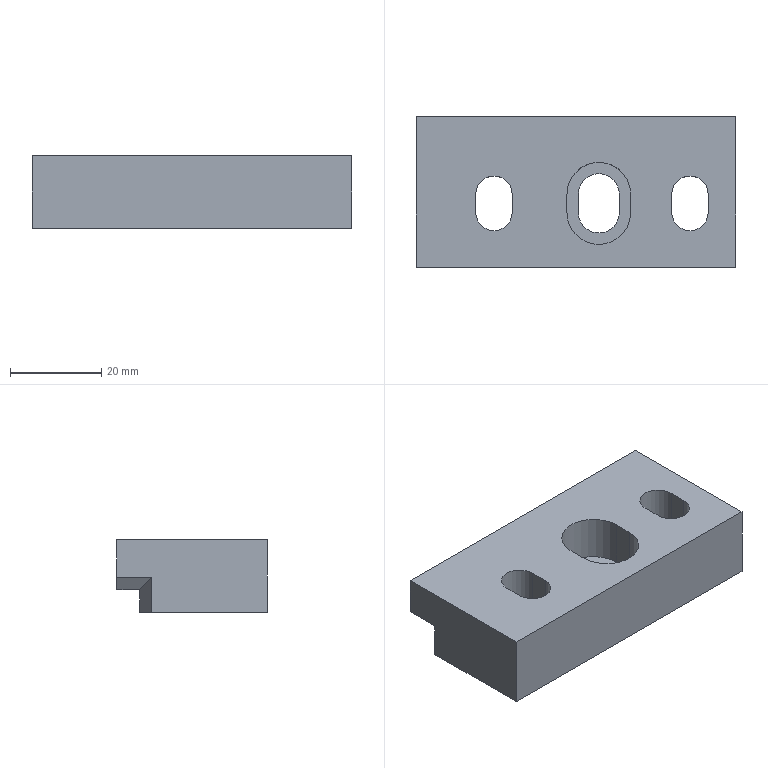Part | STEP file | 1 solid | 29 faces | box 70 x 33 x 16 mm | volume 29565 mm3 | plane 21 | cylinder 8 | commonest cylinder face diameters 8 x4 9 x2 14 x2
STEP:
#1=CARTESIAN_POINT('',(-300.,-103.979,-2.));
#2=VERTEX_POINT('',#1);
#3=CARTESIAN_POINT('',(-300.,-103.979,5.679));
#4=VERTEX_POINT('',#3);
#5=CARTESIAN_POINT('',(-300.,-103.979,-18.));
#6=DIRECTION('',(0.,0.,1.));
#7=VECTOR('',#6,1.);
#8=LINE('',#5,#7);
#9=EDGE_CURVE('',#2,#4,#8,.T.);
#10=ORIENTED_EDGE('',*,*,#9,.T.);
#11=CARTESIAN_POINT('',(-300.,-96.3,5.679));
#12=VERTEX_POINT('',#11);
#13=CARTESIAN_POINT('',(-300.,-129.3,5.679));
#14=DIRECTION('',(0.,1.,0.));
#15=VECTOR('',#14,1.);
#16=LINE('',#13,#15);
#17=EDGE_CURVE('',#4,#12,#16,.T.);
#18=ORIENTED_EDGE('',*,*,#17,.T.);
#19=CARTESIAN_POINT('',(-300.,-96.3,14.));
#20=VERTEX_POINT('',#19);
#21=CARTESIAN_POINT('',(-300.,-96.3,-2.));
#22=DIRECTION('',(0.,0.,1.));
#23=VECTOR('',#22,1.);
#24=LINE('',#21,#23);
#25=EDGE_CURVE('',#12,#20,#24,.T.);
#26=ORIENTED_EDGE('',*,*,#25,.T.);
#27=CARTESIAN_POINT('',(-300.,-129.3,14.));
#28=VERTEX_POINT('',#27);
#29=CARTESIAN_POINT('',(-300.,-129.3,14.));
#30=DIRECTION('',(0.,1.,0.));
#31=VECTOR('',#30,1.);
#32=LINE('',#29,#31);
#33=EDGE_CURVE('',#28,#20,#32,.T.);
#34=ORIENTED_EDGE('',*,*,#33,.F.);
#35=CARTESIAN_POINT('',(-300.,-129.3,-2.));
#36=VERTEX_POINT('',#35);
#37=CARTESIAN_POINT('',(-300.,-129.3,-2.));
#38=DIRECTION('',(0.,0.,1.));
#39=VECTOR('',#38,1.);
#40=LINE('',#37,#39);
#41=EDGE_CURVE('',#36,#28,#40,.T.);
#42=ORIENTED_EDGE('',*,*,#41,.F.);
#43=CARTESIAN_POINT('',(-300.,-129.3,-2.));
#44=DIRECTION('',(0.,1.,0.));
#45=VECTOR('',#44,1.);
#46=LINE('',#43,#45);
#47=EDGE_CURVE('',#36,#2,#46,.T.);
#48=ORIENTED_EDGE('',*,*,#47,.T.);
#49=EDGE_LOOP('',(#10,#18,#26,#34,#42,#48));
#50=FACE_OUTER_BOUND('',#49,.T.);
#51=CARTESIAN_POINT('',(-300.,-129.3,-2.));
#52=DIRECTION('',(1.,0.,0.));
#53=DIRECTION('',(0.,0.,-1.));
#54=AXIS2_PLACEMENT_3D('',#51,#52,#53);
#55=PLANE('',#54);
#56=ADVANCED_FACE('',(#50),#55,.T.);
#57=CARTESIAN_POINT('',(-370.,-96.3,5.679));
#58=VERTEX_POINT('',#57);
#59=CARTESIAN_POINT('',(-370.,-96.3,14.));
#60=VERTEX_POINT('',#59);
#61=CARTESIAN_POINT('',(-370.,-96.3,-2.));
#62=DIRECTION('',(0.,0.,1.));
#63=VECTOR('',#62,1.);
#64=LINE('',#61,#63);
#65=EDGE_CURVE('',#58,#60,#64,.T.);
#66=ORIENTED_EDGE('',*,*,#65,.F.);
#67=CARTESIAN_POINT('',(-370.,-103.98,5.679));
#68=VERTEX_POINT('',#67);
#69=CARTESIAN_POINT('',(-370.,-96.3,5.679));
#70=DIRECTION('',(0.,-1.,0.));
#71=VECTOR('',#70,1.);
#72=LINE('',#69,#71);
#73=EDGE_CURVE('',#58,#68,#72,.T.);
#74=ORIENTED_EDGE('',*,*,#73,.T.);
#75=CARTESIAN_POINT('',(-370.,-103.98,-2.));
#76=VERTEX_POINT('',#75);
#77=CARTESIAN_POINT('',(-370.,-103.98,-18.));
#78=DIRECTION('',(0.,0.,1.));
#79=VECTOR('',#78,1.);
#80=LINE('',#77,#79);
#81=EDGE_CURVE('',#76,#68,#80,.T.);
#82=ORIENTED_EDGE('',*,*,#81,.F.);
#83=CARTESIAN_POINT('',(-370.,-129.3,-2.));
#84=VERTEX_POINT('',#83);
#85=CARTESIAN_POINT('',(-370.,-96.3,-2.));
#86=DIRECTION('',(0.,-1.,0.));
#87=VECTOR('',#86,1.);
#88=LINE('',#85,#87);
#89=EDGE_CURVE('',#76,#84,#88,.T.);
#90=ORIENTED_EDGE('',*,*,#89,.T.);
#91=CARTESIAN_POINT('',(-370.,-129.3,14.));
#92=VERTEX_POINT('',#91);
#93=CARTESIAN_POINT('',(-370.,-129.3,-2.));
#94=DIRECTION('',(0.,0.,1.));
#95=VECTOR('',#94,1.);
#96=LINE('',#93,#95);
#97=EDGE_CURVE('',#84,#92,#96,.T.);
#98=ORIENTED_EDGE('',*,*,#97,.T.);
#99=CARTESIAN_POINT('',(-370.,-96.3,14.));
#100=DIRECTION('',(0.,-1.,0.));
#101=VECTOR('',#100,1.);
#102=LINE('',#99,#101);
#103=EDGE_CURVE('',#60,#92,#102,.T.);
#104=ORIENTED_EDGE('',*,*,#103,.F.);
#105=EDGE_LOOP('',(#66,#74,#82,#90,#98,#104));
#106=FACE_OUTER_BOUND('',#105,.T.);
#107=CARTESIAN_POINT('',(-370.,-96.3,-2.));
#108=DIRECTION('',(-1.,0.,0.));
#109=DIRECTION('',(0.,0.,1.));
#110=AXIS2_PLACEMENT_3D('',#107,#108,#109);
#111=PLANE('',#110);
#112=ADVANCED_FACE('',(#106),#111,.T.);
#113=CARTESIAN_POINT('',(-334.5,-113.3,-2.));
#114=VERTEX_POINT('',#113);
#115=CARTESIAN_POINT('',(-325.5,-113.3,-2.));
#116=VERTEX_POINT('',#115);
#117=CARTESIAN_POINT('',(-330.,-113.3,-2.));
#118=DIRECTION('',(0.,0.,-1.));
#119=DIRECTION('',(1.,0.,0.));
#120=AXIS2_PLACEMENT_3D('',#117,#118,#119);
#121=CIRCLE('',#120,4.5);
#122=EDGE_CURVE('',#114,#116,#121,.T.);
#123=ORIENTED_EDGE('',*,*,#122,.F.);
#124=CARTESIAN_POINT('',(-334.5,-117.3,-2.));
#125=VERTEX_POINT('',#124);
#126=CARTESIAN_POINT('',(-334.5,-120.3,-2.));
#127=DIRECTION('',(0.,1.,0.));
#128=VECTOR('',#127,1.);
#129=LINE('',#126,#128);
#130=EDGE_CURVE('',#125,#114,#129,.T.);
#131=ORIENTED_EDGE('',*,*,#130,.F.);
#132=CARTESIAN_POINT('',(-325.5,-117.3,-2.));
#133=VERTEX_POINT('',#132);
#134=CARTESIAN_POINT('',(-330.,-117.3,-2.));
#135=DIRECTION('',(0.,0.,-1.));
#136=DIRECTION('',(1.,0.,0.));
#137=AXIS2_PLACEMENT_3D('',#134,#135,#136);
#138=CIRCLE('',#137,4.5);
#139=EDGE_CURVE('',#133,#125,#138,.T.);
#140=ORIENTED_EDGE('',*,*,#139,.F.);
#141=CARTESIAN_POINT('',(-325.5,-113.3,-2.));
#142=DIRECTION('',(0.,-1.,0.));
#143=VECTOR('',#142,1.);
#144=LINE('',#141,#143);
#145=EDGE_CURVE('',#116,#133,#144,.T.);
#146=ORIENTED_EDGE('',*,*,#145,.F.);
#147=EDGE_LOOP('',(#123,#131,#140,#146));
#148=FACE_BOUND('',#147,.T.);
#149=CARTESIAN_POINT('',(-306.,-117.3,-2.));
#150=VERTEX_POINT('',#149);
#151=CARTESIAN_POINT('',(-306.,-113.3,-2.));
#152=VERTEX_POINT('',#151);
#153=CARTESIAN_POINT('',(-306.,-120.3,-2.));
#154=DIRECTION('',(0.,1.,0.));
#155=VECTOR('',#154,1.);
#156=LINE('',#153,#155);
#157=EDGE_CURVE('',#150,#152,#156,.T.);
#158=ORIENTED_EDGE('',*,*,#157,.T.);
#159=CARTESIAN_POINT('',(-314.,-113.3,-2.));
#160=VERTEX_POINT('',#159);
#161=CARTESIAN_POINT('',(-310.,-113.3,-2.));
#162=DIRECTION('',(0.,0.,1.));
#163=DIRECTION('',(1.,0.,0.));
#164=AXIS2_PLACEMENT_3D('',#161,#162,#163);
#165=CIRCLE('',#164,4.);
#166=EDGE_CURVE('',#152,#160,#165,.T.);
#167=ORIENTED_EDGE('',*,*,#166,.T.);
#168=CARTESIAN_POINT('',(-314.,-117.3,-2.));
#169=VERTEX_POINT('',#168);
#170=CARTESIAN_POINT('',(-314.,-113.3,-2.));
#171=DIRECTION('',(0.,-1.,0.));
#172=VECTOR('',#171,1.);
#173=LINE('',#170,#172);
#174=EDGE_CURVE('',#160,#169,#173,.T.);
#175=ORIENTED_EDGE('',*,*,#174,.T.);
#176=CARTESIAN_POINT('',(-310.,-117.3,-2.));
#177=DIRECTION('',(0.,0.,1.));
#178=DIRECTION('',(1.,0.,0.));
#179=AXIS2_PLACEMENT_3D('',#176,#177,#178);
#180=CIRCLE('',#179,4.);
#181=EDGE_CURVE('',#169,#150,#180,.T.);
#182=ORIENTED_EDGE('',*,*,#181,.T.);
#183=EDGE_LOOP('',(#158,#167,#175,#182));
#184=FACE_BOUND('',#183,.T.);
#185=CARTESIAN_POINT('',(-357.,-113.3,-2.));
#186=VERTEX_POINT('',#185);
#187=CARTESIAN_POINT('',(-349.,-113.3,-2.));
#188=VERTEX_POINT('',#187);
#189=CARTESIAN_POINT('',(-353.,-113.3,-2.));
#190=DIRECTION('',(0.,0.,-1.));
#191=DIRECTION('',(1.,0.,0.));
#192=AXIS2_PLACEMENT_3D('',#189,#190,#191);
#193=CIRCLE('',#192,4.);
#194=EDGE_CURVE('',#186,#188,#193,.T.);
#195=ORIENTED_EDGE('',*,*,#194,.F.);
#196=CARTESIAN_POINT('',(-357.,-117.3,-2.));
#197=VERTEX_POINT('',#196);
#198=CARTESIAN_POINT('',(-357.,-120.3,-2.));
#199=DIRECTION('',(0.,1.,0.));
#200=VECTOR('',#199,1.);
#201=LINE('',#198,#200);
#202=EDGE_CURVE('',#197,#186,#201,.T.);
#203=ORIENTED_EDGE('',*,*,#202,.F.);
#204=CARTESIAN_POINT('',(-349.,-117.3,-2.));
#205=VERTEX_POINT('',#204);
#206=CARTESIAN_POINT('',(-353.,-117.3,-2.));
#207=DIRECTION('',(0.,0.,-1.));
#208=DIRECTION('',(1.,0.,0.));
#209=AXIS2_PLACEMENT_3D('',#206,#207,#208);
#210=CIRCLE('',#209,4.);
#211=EDGE_CURVE('',#205,#197,#210,.T.);
#212=ORIENTED_EDGE('',*,*,#211,.F.);
#213=CARTESIAN_POINT('',(-349.,-113.3,-2.));
#214=DIRECTION('',(0.,-1.,0.));
#215=VECTOR('',#214,1.);
#216=LINE('',#213,#215);
#217=EDGE_CURVE('',#188,#205,#216,.T.);
#218=ORIENTED_EDGE('',*,*,#217,.F.);
#219=EDGE_LOOP('',(#195,#203,#212,#218));
#220=FACE_BOUND('',#219,.T.);
#221=CARTESIAN_POINT('',(-359.998,-101.3,-2.));
#222=VERTEX_POINT('',#221);
#223=CARTESIAN_POINT('',(-309.999,-101.3,-2.));
#224=VERTEX_POINT('',#223);
#225=CARTESIAN_POINT('',(-400.,-101.3,-2.));
#226=DIRECTION('',(1.,0.,0.));
#227=VECTOR('',#226,1.);
#228=LINE('',#225,#227);
#229=EDGE_CURVE('',#222,#224,#228,.T.);
#230=ORIENTED_EDGE('',*,*,#229,.T.);
#231=CARTESIAN_POINT('',(-368.146,-85.72,-2.));
#232=DIRECTION('',(-0.9659,0.2588,0.));
#233=VECTOR('',#232,1.);
#234=LINE('',#231,#233);
#235=EDGE_CURVE('',#2,#224,#234,.T.);
#236=ORIENTED_EDGE('',*,*,#235,.F.);
#237=ORIENTED_EDGE('',*,*,#47,.F.);
#238=CARTESIAN_POINT('',(-425.,-129.3,-2.));
#239=DIRECTION('',(1.,0.,0.));
#240=VECTOR('',#239,1.);
#241=LINE('',#238,#240);
#242=EDGE_CURVE('',#84,#36,#241,.T.);
#243=ORIENTED_EDGE('',*,*,#242,.F.);
#244=ORIENTED_EDGE('',*,*,#89,.F.);
#245=CARTESIAN_POINT('',(-348.505,-98.22,-2.));
#246=DIRECTION('',(0.9659,0.2588,0.));
#247=VECTOR('',#246,1.);
#248=LINE('',#245,#247);
#249=EDGE_CURVE('',#76,#222,#248,.T.);
#250=ORIENTED_EDGE('',*,*,#249,.T.);
#251=EDGE_LOOP('',(#230,#236,#237,#243,#244,#250));
#252=FACE_BOUND('',#251,.T.);
#253=CARTESIAN_POINT('',(-400.,-111.3,-2.));
#254=DIRECTION('',(0.,0.,-1.));
#255=DIRECTION('',(-1.,0.,0.));
#256=AXIS2_PLACEMENT_3D('',#253,#254,#255);
#257=PLANE('',#256);
#258=ADVANCED_FACE('',(#148,#184,#220,#252),#257,.T.);
#259=ORIENTED_EDGE('',*,*,#33,.T.);
#260=CARTESIAN_POINT('',(-325.,-96.3,14.));
#261=DIRECTION('',(-1.,0.,0.));
#262=VECTOR('',#261,1.);
#263=LINE('',#260,#262);
#264=EDGE_CURVE('',#20,#60,#263,.T.);
#265=ORIENTED_EDGE('',*,*,#264,.T.);
#266=ORIENTED_EDGE('',*,*,#103,.T.);
#267=CARTESIAN_POINT('',(-425.,-129.3,14.));
#268=DIRECTION('',(1.,0.,0.));
#269=VECTOR('',#268,1.);
#270=LINE('',#267,#269);
#271=EDGE_CURVE('',#92,#28,#270,.T.);
#272=ORIENTED_EDGE('',*,*,#271,.T.);
#273=EDGE_LOOP('',(#259,#265,#266,#272));
#274=FACE_BOUND('',#273,.T.);
#275=CARTESIAN_POINT('',(-306.,-117.3,14.));
#276=VERTEX_POINT('',#275);
#277=CARTESIAN_POINT('',(-306.,-113.3,14.));
#278=VERTEX_POINT('',#277);
#279=CARTESIAN_POINT('',(-306.,-120.3,14.));
#280=DIRECTION('',(0.,1.,0.));
#281=VECTOR('',#280,1.);
#282=LINE('',#279,#281);
#283=EDGE_CURVE('',#276,#278,#282,.T.);
#284=ORIENTED_EDGE('',*,*,#283,.F.);
#285=CARTESIAN_POINT('',(-314.,-117.3,14.));
#286=VERTEX_POINT('',#285);
#287=CARTESIAN_POINT('',(-310.,-117.3,14.));
#288=DIRECTION('',(0.,0.,1.));
#289=DIRECTION('',(1.,0.,0.));
#290=AXIS2_PLACEMENT_3D('',#287,#288,#289);
#291=CIRCLE('',#290,4.);
#292=EDGE_CURVE('',#286,#276,#291,.T.);
#293=ORIENTED_EDGE('',*,*,#292,.F.);
#294=CARTESIAN_POINT('',(-314.,-113.3,14.));
#295=VERTEX_POINT('',#294);
#296=CARTESIAN_POINT('',(-314.,-113.3,14.));
#297=DIRECTION('',(0.,-1.,0.));
#298=VECTOR('',#297,1.);
#299=LINE('',#296,#298);
#300=EDGE_CURVE('',#295,#286,#299,.T.);
#301=ORIENTED_EDGE('',*,*,#300,.F.);
#302=CARTESIAN_POINT('',(-310.,-113.3,14.));
#303=DIRECTION('',(0.,0.,1.));
#304=DIRECTION('',(1.,0.,0.));
#305=AXIS2_PLACEMENT_3D('',#302,#303,#304);
#306=CIRCLE('',#305,4.);
#307=EDGE_CURVE('',#278,#295,#306,.T.);
#308=ORIENTED_EDGE('',*,*,#307,.F.);
#309=EDGE_LOOP('',(#284,#293,#301,#308));
#310=FACE_BOUND('',#309,.T.);
#311=CARTESIAN_POINT('',(-357.,-113.3,14.));
#312=VERTEX_POINT('',#311);
#313=CARTESIAN_POINT('',(-349.,-113.3,14.));
#314=VERTEX_POINT('',#313);
#315=CARTESIAN_POINT('',(-353.,-113.3,14.));
#316=DIRECTION('',(0.,0.,-1.));
#317=DIRECTION('',(1.,0.,0.));
#318=AXIS2_PLACEMENT_3D('',#315,#316,#317);
#319=CIRCLE('',#318,4.);
#320=EDGE_CURVE('',#312,#314,#319,.T.);
#321=ORIENTED_EDGE('',*,*,#320,.T.);
#322=CARTESIAN_POINT('',(-349.,-117.3,14.));
#323=VERTEX_POINT('',#322);
#324=CARTESIAN_POINT('',(-349.,-113.3,14.));
#325=DIRECTION('',(0.,-1.,0.));
#326=VECTOR('',#325,1.);
#327=LINE('',#324,#326);
#328=EDGE_CURVE('',#314,#323,#327,.T.);
#329=ORIENTED_EDGE('',*,*,#328,.T.);
#330=CARTESIAN_POINT('',(-357.,-117.3,14.));
#331=VERTEX_POINT('',#330);
#332=CARTESIAN_POINT('',(-353.,-117.3,14.));
#333=DIRECTION('',(0.,0.,-1.));
#334=DIRECTION('',(1.,0.,0.));
#335=AXIS2_PLACEMENT_3D('',#332,#333,#334);
#336=CIRCLE('',#335,4.);
#337=EDGE_CURVE('',#323,#331,#336,.T.);
#338=ORIENTED_EDGE('',*,*,#337,.T.);
#339=CARTESIAN_POINT('',(-357.,-120.3,14.));
#340=DIRECTION('',(0.,1.,0.));
#341=VECTOR('',#340,1.);
#342=LINE('',#339,#341);
#343=EDGE_CURVE('',#331,#312,#342,.T.);
#344=ORIENTED_EDGE('',*,*,#343,.T.);
#345=EDGE_LOOP('',(#321,#329,#338,#344));
#346=FACE_BOUND('',#345,.T.);
#347=CARTESIAN_POINT('',(-337.,-117.3,14.));
#348=VERTEX_POINT('',#347);
#349=CARTESIAN_POINT('',(-337.,-113.3,14.));
#350=VERTEX_POINT('',#349);
#351=CARTESIAN_POINT('',(-337.,-120.3,14.));
#352=DIRECTION('',(0.,1.,0.));
#353=VECTOR('',#352,1.);
#354=LINE('',#351,#353);
#355=EDGE_CURVE('',#348,#350,#354,.T.);
#356=ORIENTED_EDGE('',*,*,#355,.T.);
#357=CARTESIAN_POINT('',(-323.,-113.3,14.));
#358=VERTEX_POINT('',#357);
#359=CARTESIAN_POINT('',(-330.,-113.3,14.));
#360=DIRECTION('',(0.,0.,-1.));
#361=DIRECTION('',(1.,0.,0.));
#362=AXIS2_PLACEMENT_3D('',#359,#360,#361);
#363=CIRCLE('',#362,7.);
#364=EDGE_CURVE('',#350,#358,#363,.T.);
#365=ORIENTED_EDGE('',*,*,#364,.T.);
#366=CARTESIAN_POINT('',(-323.,-117.3,14.));
#367=VERTEX_POINT('',#366);
#368=CARTESIAN_POINT('',(-323.,-113.3,14.));
#369=DIRECTION('',(0.,-1.,0.));
#370=VECTOR('',#369,1.);
#371=LINE('',#368,#370);
#372=EDGE_CURVE('',#358,#367,#371,.T.);
#373=ORIENTED_EDGE('',*,*,#372,.T.);
#374=CARTESIAN_POINT('',(-330.,-117.3,14.));
#375=DIRECTION('',(0.,0.,-1.));
#376=DIRECTION('',(1.,0.,0.));
#377=AXIS2_PLACEMENT_3D('',#374,#375,#376);
#378=CIRCLE('',#377,7.);
#379=EDGE_CURVE('',#367,#348,#378,.T.);
#380=ORIENTED_EDGE('',*,*,#379,.T.);
#381=EDGE_LOOP('',(#356,#365,#373,#380));
#382=FACE_BOUND('',#381,.T.);
#383=CARTESIAN_POINT('',(-400.,-111.3,14.));
#384=DIRECTION('',(0.,0.,-1.));
#385=DIRECTION('',(-1.,0.,0.));
#386=AXIS2_PLACEMENT_3D('',#383,#384,#385);
#387=PLANE('',#386);
#388=ADVANCED_FACE('',(#274,#310,#346,#382),#387,.F.);
#389=CARTESIAN_POINT('',(-334.5,-113.3,4.));
#390=VERTEX_POINT('',#389);
#391=CARTESIAN_POINT('',(-325.5,-113.3,4.));
#392=VERTEX_POINT('',#391);
#393=CARTESIAN_POINT('',(-330.,-113.3,4.));
#394=DIRECTION('',(0.,0.,-1.));
#395=DIRECTION('',(-1.,0.,0.));
#396=AXIS2_PLACEMENT_3D('',#393,#394,#395);
#397=CIRCLE('',#396,4.5);
#398=EDGE_CURVE('',#390,#392,#397,.T.);
#399=ORIENTED_EDGE('',*,*,#398,.F.);
#400=CARTESIAN_POINT('',(-334.5,-113.3,-2.));
#401=DIRECTION('',(0.,0.,1.));
#402=VECTOR('',#401,1.);
#403=LINE('',#400,#402);
#404=EDGE_CURVE('',#114,#390,#403,.T.);
#405=ORIENTED_EDGE('',*,*,#404,.F.);
#406=ORIENTED_EDGE('',*,*,#122,.T.);
#407=CARTESIAN_POINT('',(-325.5,-113.3,-2.));
#408=DIRECTION('',(0.,0.,1.));
#409=VECTOR('',#408,1.);
#410=LINE('',#407,#409);
#411=EDGE_CURVE('',#116,#392,#410,.T.);
#412=ORIENTED_EDGE('',*,*,#411,.T.);
#413=EDGE_LOOP('',(#399,#405,#406,#412));
#414=FACE_OUTER_BOUND('',#413,.T.);
#415=CARTESIAN_POINT('',(-330.,-113.3,-2.));
#416=DIRECTION('',(0.,0.,1.));
#417=DIRECTION('',(1.,0.,0.));
#418=AXIS2_PLACEMENT_3D('',#415,#416,#417);
#419=CYLINDRICAL_SURFACE('',#418,4.5);
#420=ADVANCED_FACE('',(#414),#419,.F.);
#421=CARTESIAN_POINT('',(-325.5,-117.3,4.));
#422=VERTEX_POINT('',#421);
#423=CARTESIAN_POINT('',(-325.5,-113.3,4.));
#424=DIRECTION('',(0.,-1.,0.));
#425=VECTOR('',#424,1.);
#426=LINE('',#423,#425);
#427=EDGE_CURVE('',#392,#422,#426,.T.);
#428=ORIENTED_EDGE('',*,*,#427,.F.);
#429=ORIENTED_EDGE('',*,*,#411,.F.);
#430=ORIENTED_EDGE('',*,*,#145,.T.);
#431=CARTESIAN_POINT('',(-325.5,-117.3,-2.));
#432=DIRECTION('',(0.,0.,1.));
#433=VECTOR('',#432,1.);
#434=LINE('',#431,#433);
#435=EDGE_CURVE('',#133,#422,#434,.T.);
#436=ORIENTED_EDGE('',*,*,#435,.T.);
#437=EDGE_LOOP('',(#428,#429,#430,#436));
#438=FACE_OUTER_BOUND('',#437,.T.);
#439=CARTESIAN_POINT('',(-325.5,-113.3,-2.));
#440=DIRECTION('',(-1.,0.,0.));
#441=DIRECTION('',(0.,0.,1.));
#442=AXIS2_PLACEMENT_3D('',#439,#440,#441);
#443=PLANE('',#442);
#444=ADVANCED_FACE('',(#438),#443,.T.);
#445=CARTESIAN_POINT('',(-334.5,-117.3,4.));
#446=VERTEX_POINT('',#445);
#447=CARTESIAN_POINT('',(-330.,-117.3,4.));
#448=DIRECTION('',(0.,0.,-1.));
#449=DIRECTION('',(-1.,0.,0.));
#450=AXIS2_PLACEMENT_3D('',#447,#448,#449);
#451=CIRCLE('',#450,4.5);
#452=EDGE_CURVE('',#422,#446,#451,.T.);
#453=ORIENTED_EDGE('',*,*,#452,.F.);
#454=ORIENTED_EDGE('',*,*,#435,.F.);
#455=ORIENTED_EDGE('',*,*,#139,.T.);
#456=CARTESIAN_POINT('',(-334.5,-117.3,-2.));
#457=DIRECTION('',(0.,0.,1.));
#458=VECTOR('',#457,1.);
#459=LINE('',#456,#458);
#460=EDGE_CURVE('',#125,#446,#459,.T.);
#461=ORIENTED_EDGE('',*,*,#460,.T.);
#462=EDGE_LOOP('',(#453,#454,#455,#461));
#463=FACE_OUTER_BOUND('',#462,.T.);
#464=CARTESIAN_POINT('',(-330.,-117.3,-2.));
#465=DIRECTION('',(0.,0.,1.));
#466=DIRECTION('',(1.,0.,0.));
#467=AXIS2_PLACEMENT_3D('',#464,#465,#466);
#468=CYLINDRICAL_SURFACE('',#467,4.5);
#469=ADVANCED_FACE('',(#463),#468,.F.);
#470=ORIENTED_EDGE('',*,*,#283,.T.);
#471=CARTESIAN_POINT('',(-306.,-113.3,-2.));
#472=DIRECTION('',(0.,0.,1.));
#473=VECTOR('',#472,1.);
#474=LINE('',#471,#473);
#475=EDGE_CURVE('',#152,#278,#474,.T.);
#476=ORIENTED_EDGE('',*,*,#475,.F.);
#477=ORIENTED_EDGE('',*,*,#157,.F.);
#478=CARTESIAN_POINT('',(-306.,-117.3,-2.));
#479=DIRECTION('',(0.,0.,1.));
#480=VECTOR('',#479,1.);
#481=LINE('',#478,#480);
#482=EDGE_CURVE('',#150,#276,#481,.T.);
#483=ORIENTED_EDGE('',*,*,#482,.T.);
#484=EDGE_LOOP('',(#470,#476,#477,#483));
#485=FACE_OUTER_BOUND('',#484,.T.);
#486=CARTESIAN_POINT('',(-306.,-120.3,-2.));
#487=DIRECTION('',(1.,0.,0.));
#488=DIRECTION('',(0.,0.,-1.));
#489=AXIS2_PLACEMENT_3D('',#486,#487,#488);
#490=PLANE('',#489);
#491=ADVANCED_FACE('',(#485),#490,.F.);
#492=ORIENTED_EDGE('',*,*,#292,.T.);
#493=ORIENTED_EDGE('',*,*,#482,.F.);
#494=ORIENTED_EDGE('',*,*,#181,.F.);
#495=CARTESIAN_POINT('',(-314.,-117.3,-2.));
#496=DIRECTION('',(0.,0.,1.));
#497=VECTOR('',#496,1.);
#498=LINE('',#495,#497);
#499=EDGE_CURVE('',#169,#286,#498,.T.);
#500=ORIENTED_EDGE('',*,*,#499,.T.);
#501=EDGE_LOOP('',(#492,#493,#494,#500));
#502=FACE_OUTER_BOUND('',#501,.T.);
#503=CARTESIAN_POINT('',(-310.,-117.3,-2.));
#504=DIRECTION('',(0.,0.,1.));
#505=DIRECTION('',(1.,0.,0.));
#506=AXIS2_PLACEMENT_3D('',#503,#504,#505);
#507=CYLINDRICAL_SURFACE('',#506,4.);
#508=ADVANCED_FACE('',(#502),#507,.F.);
#509=ORIENTED_EDGE('',*,*,#300,.T.);
#510=ORIENTED_EDGE('',*,*,#499,.F.);
#511=ORIENTED_EDGE('',*,*,#174,.F.);
#512=CARTESIAN_POINT('',(-314.,-113.3,-2.));
#513=DIRECTION('',(0.,0.,1.));
#514=VECTOR('',#513,1.);
#515=LINE('',#512,#514);
#516=EDGE_CURVE('',#160,#295,#515,.T.);
#517=ORIENTED_EDGE('',*,*,#516,.T.);
#518=EDGE_LOOP('',(#509,#510,#511,#517));
#519=FACE_OUTER_BOUND('',#518,.T.);
#520=CARTESIAN_POINT('',(-314.,-113.3,-2.));
#521=DIRECTION('',(-1.,0.,0.));
#522=DIRECTION('',(0.,0.,1.));
#523=AXIS2_PLACEMENT_3D('',#520,#521,#522);
#524=PLANE('',#523);
#525=ADVANCED_FACE('',(#519),#524,.F.);
#526=ORIENTED_EDGE('',*,*,#320,.F.);
#527=CARTESIAN_POINT('',(-357.,-113.3,-2.));
#528=DIRECTION('',(0.,0.,1.));
#529=VECTOR('',#528,1.);
#530=LINE('',#527,#529);
#531=EDGE_CURVE('',#186,#312,#530,.T.);
#532=ORIENTED_EDGE('',*,*,#531,.F.);
#533=ORIENTED_EDGE('',*,*,#194,.T.);
#534=CARTESIAN_POINT('',(-349.,-113.3,-2.));
#535=DIRECTION('',(0.,0.,1.));
#536=VECTOR('',#535,1.);
#537=LINE('',#534,#536);
#538=EDGE_CURVE('',#188,#314,#537,.T.);
#539=ORIENTED_EDGE('',*,*,#538,.T.);
#540=EDGE_LOOP('',(#526,#532,#533,#539));
#541=FACE_OUTER_BOUND('',#540,.T.);
#542=CARTESIAN_POINT('',(-353.,-113.3,-2.));
#543=DIRECTION('',(0.,0.,1.));
#544=DIRECTION('',(1.,0.,0.));
#545=AXIS2_PLACEMENT_3D('',#542,#543,#544);
#546=CYLINDRICAL_SURFACE('',#545,4.);
#547=ADVANCED_FACE('',(#541),#546,.F.);
#548=ORIENTED_EDGE('',*,*,#328,.F.);
#549=ORIENTED_EDGE('',*,*,#538,.F.);
#550=ORIENTED_EDGE('',*,*,#217,.T.);
#551=CARTESIAN_POINT('',(-349.,-117.3,-2.));
#552=DIRECTION('',(0.,0.,1.));
#553=VECTOR('',#552,1.);
#554=LINE('',#551,#553);
#555=EDGE_CURVE('',#205,#323,#554,.T.);
#556=ORIENTED_EDGE('',*,*,#555,.T.);
#557=EDGE_LOOP('',(#548,#549,#550,#556));
#558=FACE_OUTER_BOUND('',#557,.T.);
#559=CARTESIAN_POINT('',(-349.,-113.3,-2.));
#560=DIRECTION('',(-1.,0.,0.));
#561=DIRECTION('',(0.,0.,1.));
#562=AXIS2_PLACEMENT_3D('',#559,#560,#561);
#563=PLANE('',#562);
#564=ADVANCED_FACE('',(#558),#563,.T.);
#565=ORIENTED_EDGE('',*,*,#337,.F.);
#566=ORIENTED_EDGE('',*,*,#555,.F.);
#567=ORIENTED_EDGE('',*,*,#211,.T.);
#568=CARTESIAN_POINT('',(-357.,-117.3,-2.));
#569=DIRECTION('',(0.,0.,1.));
#570=VECTOR('',#569,1.);
#571=LINE('',#568,#570);
#572=EDGE_CURVE('',#197,#331,#571,.T.);
#573=ORIENTED_EDGE('',*,*,#572,.T.);
#574=EDGE_LOOP('',(#565,#566,#567,#573));
#575=FACE_OUTER_BOUND('',#574,.T.);
#576=CARTESIAN_POINT('',(-353.,-117.3,-2.));
#577=DIRECTION('',(0.,0.,1.));
#578=DIRECTION('',(1.,0.,0.));
#579=AXIS2_PLACEMENT_3D('',#576,#577,#578);
#580=CYLINDRICAL_SURFACE('',#579,4.);
#581=ADVANCED_FACE('',(#575),#580,.F.);
#582=CARTESIAN_POINT('',(-334.5,-120.3,4.));
#583=DIRECTION('',(0.,1.,0.));
#584=VECTOR('',#583,1.);
#585=LINE('',#582,#584);
#586=EDGE_CURVE('',#446,#390,#585,.T.);
#587=ORIENTED_EDGE('',*,*,#586,.F.);
#588=ORIENTED_EDGE('',*,*,#460,.F.);
#589=ORIENTED_EDGE('',*,*,#130,.T.);
#590=ORIENTED_EDGE('',*,*,#404,.T.);
#591=EDGE_LOOP('',(#587,#588,#589,#590));
#592=FACE_OUTER_BOUND('',#591,.T.);
#593=CARTESIAN_POINT('',(-334.5,-120.3,-2.));
#594=DIRECTION('',(1.,0.,0.));
#595=DIRECTION('',(0.,0.,-1.));
#596=AXIS2_PLACEMENT_3D('',#593,#594,#595);
#597=PLANE('',#596);
#598=ADVANCED_FACE('',(#592),#597,.T.);
#599=ORIENTED_EDGE('',*,*,#307,.T.);
#600=ORIENTED_EDGE('',*,*,#516,.F.);
#601=ORIENTED_EDGE('',*,*,#166,.F.);
#602=ORIENTED_EDGE('',*,*,#475,.T.);
#603=EDGE_LOOP('',(#599,#600,#601,#602));
#604=FACE_OUTER_BOUND('',#603,.T.);
#605=CARTESIAN_POINT('',(-310.,-113.3,-2.));
#606=DIRECTION('',(0.,0.,1.));
#607=DIRECTION('',(1.,0.,0.));
#608=AXIS2_PLACEMENT_3D('',#605,#606,#607);
#609=CYLINDRICAL_SURFACE('',#608,4.);
#610=ADVANCED_FACE('',(#604),#609,.F.);
#611=ORIENTED_EDGE('',*,*,#343,.F.);
#612=ORIENTED_EDGE('',*,*,#572,.F.);
#613=ORIENTED_EDGE('',*,*,#202,.T.);
#614=ORIENTED_EDGE('',*,*,#531,.T.);
#615=EDGE_LOOP('',(#611,#612,#613,#614));
#616=FACE_OUTER_BOUND('',#615,.T.);
#617=CARTESIAN_POINT('',(-357.,-120.3,-2.));
#618=DIRECTION('',(1.,0.,0.));
#619=DIRECTION('',(0.,0.,-1.));
#620=AXIS2_PLACEMENT_3D('',#617,#618,#619);
#621=PLANE('',#620);
#622=ADVANCED_FACE('',(#616),#621,.T.);
#623=ORIENTED_EDGE('',*,*,#271,.F.);
#624=ORIENTED_EDGE('',*,*,#97,.F.);
#625=ORIENTED_EDGE('',*,*,#242,.T.);
#626=ORIENTED_EDGE('',*,*,#41,.T.);
#627=EDGE_LOOP('',(#623,#624,#625,#626));
#628=FACE_OUTER_BOUND('',#627,.T.);
#629=CARTESIAN_POINT('',(-425.,-129.3,-2.));
#630=DIRECTION('',(0.,-1.,0.));
#631=DIRECTION('',(0.,0.,-1.));
#632=AXIS2_PLACEMENT_3D('',#629,#630,#631);
#633=PLANE('',#632);
#634=ADVANCED_FACE('',(#628),#633,.T.);
#635=ORIENTED_EDGE('',*,*,#364,.F.);
#636=CARTESIAN_POINT('',(-337.,-113.3,4.));
#637=VERTEX_POINT('',#636);
#638=CARTESIAN_POINT('',(-337.,-113.3,4.));
#639=DIRECTION('',(0.,0.,-1.));
#640=VECTOR('',#639,1.);
#641=LINE('',#638,#640);
#642=EDGE_CURVE('',#350,#637,#641,.T.);
#643=ORIENTED_EDGE('',*,*,#642,.T.);
#644=CARTESIAN_POINT('',(-323.,-113.3,4.));
#645=VERTEX_POINT('',#644);
#646=CARTESIAN_POINT('',(-330.,-113.3,4.));
#647=DIRECTION('',(0.,0.,1.));
#648=DIRECTION('',(1.,0.,0.));
#649=AXIS2_PLACEMENT_3D('',#646,#647,#648);
#650=CIRCLE('',#649,7.);
#651=EDGE_CURVE('',#645,#637,#650,.T.);
#652=ORIENTED_EDGE('',*,*,#651,.F.);
#653=CARTESIAN_POINT('',(-323.,-113.3,4.));
#654=DIRECTION('',(0.,0.,-1.));
#655=VECTOR('',#654,1.);
#656=LINE('',#653,#655);
#657=EDGE_CURVE('',#358,#645,#656,.T.);
#658=ORIENTED_EDGE('',*,*,#657,.F.);
#659=EDGE_LOOP('',(#635,#643,#652,#658));
#660=FACE_OUTER_BOUND('',#659,.T.);
#661=CARTESIAN_POINT('',(-330.,-113.3,4.));
#662=DIRECTION('',(0.,0.,1.));
#663=DIRECTION('',(1.,0.,0.));
#664=AXIS2_PLACEMENT_3D('',#661,#662,#663);
#665=CYLINDRICAL_SURFACE('',#664,7.);
#666=ADVANCED_FACE('',(#660),#665,.F.);
#667=ORIENTED_EDGE('',*,*,#372,.F.);
#668=ORIENTED_EDGE('',*,*,#657,.T.);
#669=CARTESIAN_POINT('',(-323.,-117.3,4.));
#670=VERTEX_POINT('',#669);
#671=CARTESIAN_POINT('',(-323.,-113.3,4.));
#672=DIRECTION('',(0.,1.,0.));
#673=VECTOR('',#672,1.);
#674=LINE('',#671,#673);
#675=EDGE_CURVE('',#670,#645,#674,.T.);
#676=ORIENTED_EDGE('',*,*,#675,.F.);
#677=CARTESIAN_POINT('',(-323.,-117.3,4.));
#678=DIRECTION('',(0.,0.,-1.));
#679=VECTOR('',#678,1.);
#680=LINE('',#677,#679);
#681=EDGE_CURVE('',#367,#670,#680,.T.);
#682=ORIENTED_EDGE('',*,*,#681,.F.);
#683=EDGE_LOOP('',(#667,#668,#676,#682));
#684=FACE_OUTER_BOUND('',#683,.T.);
#685=CARTESIAN_POINT('',(-323.,-113.3,4.));
#686=DIRECTION('',(-1.,0.,0.));
#687=DIRECTION('',(0.,0.,1.));
#688=AXIS2_PLACEMENT_3D('',#685,#686,#687);
#689=PLANE('',#688);
#690=ADVANCED_FACE('',(#684),#689,.T.);
#691=ORIENTED_EDGE('',*,*,#379,.F.);
#692=ORIENTED_EDGE('',*,*,#681,.T.);
#693=CARTESIAN_POINT('',(-337.,-117.3,4.));
#694=VERTEX_POINT('',#693);
#695=CARTESIAN_POINT('',(-330.,-117.3,4.));
#696=DIRECTION('',(0.,0.,1.));
#697=DIRECTION('',(1.,0.,0.));
#698=AXIS2_PLACEMENT_3D('',#695,#696,#697);
#699=CIRCLE('',#698,7.);
#700=EDGE_CURVE('',#694,#670,#699,.T.);
#701=ORIENTED_EDGE('',*,*,#700,.F.);
#702=CARTESIAN_POINT('',(-337.,-117.3,4.));
#703=DIRECTION('',(0.,0.,-1.));
#704=VECTOR('',#703,1.);
#705=LINE('',#702,#704);
#706=EDGE_CURVE('',#348,#694,#705,.T.);
#707=ORIENTED_EDGE('',*,*,#706,.F.);
#708=EDGE_LOOP('',(#691,#692,#701,#707));
#709=FACE_OUTER_BOUND('',#708,.T.);
#710=CARTESIAN_POINT('',(-330.,-117.3,4.));
#711=DIRECTION('',(0.,0.,1.));
#712=DIRECTION('',(1.,0.,0.));
#713=AXIS2_PLACEMENT_3D('',#710,#711,#712);
#714=CYLINDRICAL_SURFACE('',#713,7.);
#715=ADVANCED_FACE('',(#709),#714,.F.);
#716=ORIENTED_EDGE('',*,*,#355,.F.);
#717=ORIENTED_EDGE('',*,*,#706,.T.);
#718=CARTESIAN_POINT('',(-337.,-120.3,4.));
#719=DIRECTION('',(0.,-1.,0.));
#720=VECTOR('',#719,1.);
#721=LINE('',#718,#720);
#722=EDGE_CURVE('',#637,#694,#721,.T.);
#723=ORIENTED_EDGE('',*,*,#722,.F.);
#724=ORIENTED_EDGE('',*,*,#642,.F.);
#725=EDGE_LOOP('',(#716,#717,#723,#724));
#726=FACE_OUTER_BOUND('',#725,.T.);
#727=CARTESIAN_POINT('',(-337.,-120.3,4.));
#728=DIRECTION('',(1.,0.,0.));
#729=DIRECTION('',(0.,0.,-1.));
#730=AXIS2_PLACEMENT_3D('',#727,#728,#729);
#731=PLANE('',#730);
#732=ADVANCED_FACE('',(#726),#731,.T.);
#733=ORIENTED_EDGE('',*,*,#398,.T.);
#734=ORIENTED_EDGE('',*,*,#427,.T.);
#735=ORIENTED_EDGE('',*,*,#452,.T.);
#736=ORIENTED_EDGE('',*,*,#586,.T.);
#737=EDGE_LOOP('',(#733,#734,#735,#736));
#738=FACE_BOUND('',#737,.T.);
#739=ORIENTED_EDGE('',*,*,#651,.T.);
#740=ORIENTED_EDGE('',*,*,#722,.T.);
#741=ORIENTED_EDGE('',*,*,#700,.T.);
#742=ORIENTED_EDGE('',*,*,#675,.T.);
#743=EDGE_LOOP('',(#739,#740,#741,#742));
#744=FACE_BOUND('',#743,.T.);
#745=CARTESIAN_POINT('',(-330.,-113.3,4.));
#746=DIRECTION('',(0.,0.,-1.));
#747=DIRECTION('',(-1.,0.,0.));
#748=AXIS2_PLACEMENT_3D('',#745,#746,#747);
#749=PLANE('',#748);
#750=ADVANCED_FACE('',(#738,#744),#749,.F.);
#751=CARTESIAN_POINT('',(-309.999,-101.3,3.));
#752=VERTEX_POINT('',#751);
#753=CARTESIAN_POINT('',(-309.999,-101.3,-18.));
#754=DIRECTION('',(0.,0.,1.));
#755=VECTOR('',#754,1.);
#756=LINE('',#753,#755);
#757=EDGE_CURVE('',#224,#752,#756,.T.);
#758=ORIENTED_EDGE('',*,*,#757,.T.);
#759=CARTESIAN_POINT('',(-294.067,-105.569,7.269));
#760=DIRECTION('',(0.9351,-0.2506,0.2506));
#761=VECTOR('',#760,1.);
#762=LINE('',#759,#761);
#763=EDGE_CURVE('',#752,#4,#762,.T.);
#764=ORIENTED_EDGE('',*,*,#763,.T.);
#765=ORIENTED_EDGE('',*,*,#9,.F.);
#766=ORIENTED_EDGE('',*,*,#235,.T.);
#767=EDGE_LOOP('',(#758,#764,#765,#766));
#768=FACE_OUTER_BOUND('',#767,.T.);
#769=CARTESIAN_POINT('',(-300.,-103.979,-18.));
#770=DIRECTION('',(0.2588,0.9659,0.));
#771=DIRECTION('',(-0.9659,0.2588,0.));
#772=AXIS2_PLACEMENT_3D('',#769,#770,#771);
#773=PLANE('',#772);
#774=ADVANCED_FACE('',(#768),#773,.T.);
#775=CARTESIAN_POINT('',(-360.,-101.3,3.));
#776=VERTEX_POINT('',#775);
#777=CARTESIAN_POINT('',(-400.,-101.3,3.));
#778=DIRECTION('',(1.,0.,0.));
#779=VECTOR('',#778,1.);
#780=LINE('',#777,#779);
#781=EDGE_CURVE('',#776,#752,#780,.T.);
#782=ORIENTED_EDGE('',*,*,#781,.T.);
#783=ORIENTED_EDGE('',*,*,#757,.F.);
#784=ORIENTED_EDGE('',*,*,#229,.F.);
#785=CARTESIAN_POINT('',(-359.998,-101.3,-18.));
#786=DIRECTION('',(0.,0.,1.));
#787=VECTOR('',#786,1.);
#788=LINE('',#785,#787);
#789=EDGE_CURVE('',#222,#776,#788,.T.);
#790=ORIENTED_EDGE('',*,*,#789,.T.);
#791=EDGE_LOOP('',(#782,#783,#784,#790));
#792=FACE_OUTER_BOUND('',#791,.T.);
#793=CARTESIAN_POINT('',(-335.,-101.3,-18.));
#794=DIRECTION('',(0.,1.,0.));
#795=DIRECTION('',(0.,0.,1.));
#796=AXIS2_PLACEMENT_3D('',#793,#794,#795);
#797=PLANE('',#796);
#798=ADVANCED_FACE('',(#792),#797,.T.);
#799=ORIENTED_EDGE('',*,*,#81,.T.);
#800=CARTESIAN_POINT('',(-368.201,-103.498,5.197));
#801=DIRECTION('',(0.9351,0.2506,-0.2506));
#802=VECTOR('',#801,1.);
#803=LINE('',#800,#802);
#804=EDGE_CURVE('',#68,#776,#803,.T.);
#805=ORIENTED_EDGE('',*,*,#804,.T.);
#806=ORIENTED_EDGE('',*,*,#789,.F.);
#807=ORIENTED_EDGE('',*,*,#249,.F.);
#808=EDGE_LOOP('',(#799,#805,#806,#807));
#809=FACE_OUTER_BOUND('',#808,.T.);
#810=CARTESIAN_POINT('',(-360.,-101.3,-18.));
#811=DIRECTION('',(-0.2588,0.9659,0.));
#812=DIRECTION('',(-0.9659,-0.2588,0.));
#813=AXIS2_PLACEMENT_3D('',#810,#811,#812);
#814=PLANE('',#813);
#815=ADVANCED_FACE('',(#809),#814,.T.);
#816=ORIENTED_EDGE('',*,*,#25,.F.);
#817=CARTESIAN_POINT('',(-310.,-96.3,3.));
#818=VERTEX_POINT('',#817);
#819=CARTESIAN_POINT('',(-302.67,-96.3,4.964));
#820=DIRECTION('',(-0.9659,0.,-0.2588));
#821=VECTOR('',#820,1.);
#822=LINE('',#819,#821);
#823=EDGE_CURVE('',#12,#818,#822,.T.);
#824=ORIENTED_EDGE('',*,*,#823,.T.);
#825=CARTESIAN_POINT('',(-360.,-96.3,3.));
#826=VERTEX_POINT('',#825);
#827=CARTESIAN_POINT('',(-325.,-96.3,3.));
#828=DIRECTION('',(-1.,0.,0.));
#829=VECTOR('',#828,1.);
#830=LINE('',#827,#829);
#831=EDGE_CURVE('',#818,#826,#830,.T.);
#832=ORIENTED_EDGE('',*,*,#831,.T.);
#833=CARTESIAN_POINT('',(-274.029,-96.3,-20.036));
#834=DIRECTION('',(-0.9659,0.,0.2588));
#835=VECTOR('',#834,1.);
#836=LINE('',#833,#835);
#837=EDGE_CURVE('',#826,#58,#836,.T.);
#838=ORIENTED_EDGE('',*,*,#837,.T.);
#839=ORIENTED_EDGE('',*,*,#65,.T.);
#840=ORIENTED_EDGE('',*,*,#264,.F.);
#841=EDGE_LOOP('',(#816,#824,#832,#838,#839,#840));
#842=FACE_OUTER_BOUND('',#841,.T.);
#843=CARTESIAN_POINT('',(-325.,-96.3,-2.));
#844=DIRECTION('',(0.,1.,0.));
#845=DIRECTION('',(0.,0.,1.));
#846=AXIS2_PLACEMENT_3D('',#843,#844,#845);
#847=PLANE('',#846);
#848=ADVANCED_FACE('',(#842),#847,.T.);
#849=ORIENTED_EDGE('',*,*,#831,.F.);
#850=CARTESIAN_POINT('',(-310.,-111.3,3.));
#851=DIRECTION('',(0.,-1.,0.));
#852=VECTOR('',#851,1.);
#853=LINE('',#850,#852);
#854=EDGE_CURVE('',#818,#752,#853,.T.);
#855=ORIENTED_EDGE('',*,*,#854,.T.);
#856=ORIENTED_EDGE('',*,*,#781,.F.);
#857=CARTESIAN_POINT('',(-360.,-111.3,3.));
#858=DIRECTION('',(0.,1.,0.));
#859=VECTOR('',#858,1.);
#860=LINE('',#857,#859);
#861=EDGE_CURVE('',#776,#826,#860,.T.);
#862=ORIENTED_EDGE('',*,*,#861,.T.);
#863=EDGE_LOOP('',(#849,#855,#856,#862));
#864=FACE_OUTER_BOUND('',#863,.T.);
#865=CARTESIAN_POINT('',(-400.,-111.3,3.));
#866=DIRECTION('',(0.,0.,-1.));
#867=DIRECTION('',(-1.,0.,0.));
#868=AXIS2_PLACEMENT_3D('',#865,#866,#867);
#869=PLANE('',#868);
#870=ADVANCED_FACE('',(#864),#869,.T.);
#871=ORIENTED_EDGE('',*,*,#837,.F.);
#872=ORIENTED_EDGE('',*,*,#861,.F.);
#873=ORIENTED_EDGE('',*,*,#804,.F.);
#874=ORIENTED_EDGE('',*,*,#73,.F.);
#875=EDGE_LOOP('',(#871,#872,#873,#874));
#876=FACE_OUTER_BOUND('',#875,.T.);
#877=CARTESIAN_POINT('',(-370.,-96.3,5.679));
#878=DIRECTION('',(0.2588,0.,0.9659));
#879=DIRECTION('',(0.9659,0.,-0.2588));
#880=AXIS2_PLACEMENT_3D('',#877,#878,#879);
#881=PLANE('',#880);
#882=ADVANCED_FACE('',(#876),#881,.F.);
#883=ORIENTED_EDGE('',*,*,#763,.F.);
#884=ORIENTED_EDGE('',*,*,#854,.F.);
#885=ORIENTED_EDGE('',*,*,#823,.F.);
#886=ORIENTED_EDGE('',*,*,#17,.F.);
#887=EDGE_LOOP('',(#883,#884,#885,#886));
#888=FACE_OUTER_BOUND('',#887,.T.);
#889=CARTESIAN_POINT('',(-300.,-129.3,5.679));
#890=DIRECTION('',(-0.2588,0.,0.9659));
#891=DIRECTION('',(0.9659,0.,0.2588));
#892=AXIS2_PLACEMENT_3D('',#889,#890,#891);
#893=PLANE('',#892);
#894=ADVANCED_FACE('',(#888),#893,.F.);
#895=CLOSED_SHELL('',(#56,#112,#258,#388,#420,#444,#469,#491,#508,#525,#547,#564,#581,#598,#610,#622,#634,#666,#690,#715,#732,#750,#774,#798,#815,#848,#870,#882,#894));
#896=MANIFOLD_SOLID_BREP('',#895);
#897=(LENGTH_UNIT()NAMED_UNIT(*)SI_UNIT(.MILLI.,.METRE.));
#898=UNCERTAINTY_MEASURE_WITH_UNIT(LENGTH_MEASURE(0.002707),#897,'','');
#899=(NAMED_UNIT(*)PLANE_ANGLE_UNIT()SI_UNIT($,.RADIAN.));
#900=PLANE_ANGLE_MEASURE_WITH_UNIT(PLANE_ANGLE_MEASURE(0.01745),#899);
#901=DIMENSIONAL_EXPONENTS(0.,0.,0.,0.,0.,0.,0.);
#902=(CONVERSION_BASED_UNIT('DEGREE',#900)NAMED_UNIT(#901)PLANE_ANGLE_UNIT());
#903=(NAMED_UNIT(*)SI_UNIT($,.STERADIAN.)SOLID_ANGLE_UNIT());
#904=(GEOMETRIC_REPRESENTATION_CONTEXT(3)GLOBAL_UNCERTAINTY_ASSIGNED_CONTEXT((#898))GLOBAL_UNIT_ASSIGNED_CONTEXT((#897,#902,#903))REPRESENTATION_CONTEXT('',''));
#905=ADVANCED_BREP_SHAPE_REPRESENTATION('',(#896),#904);